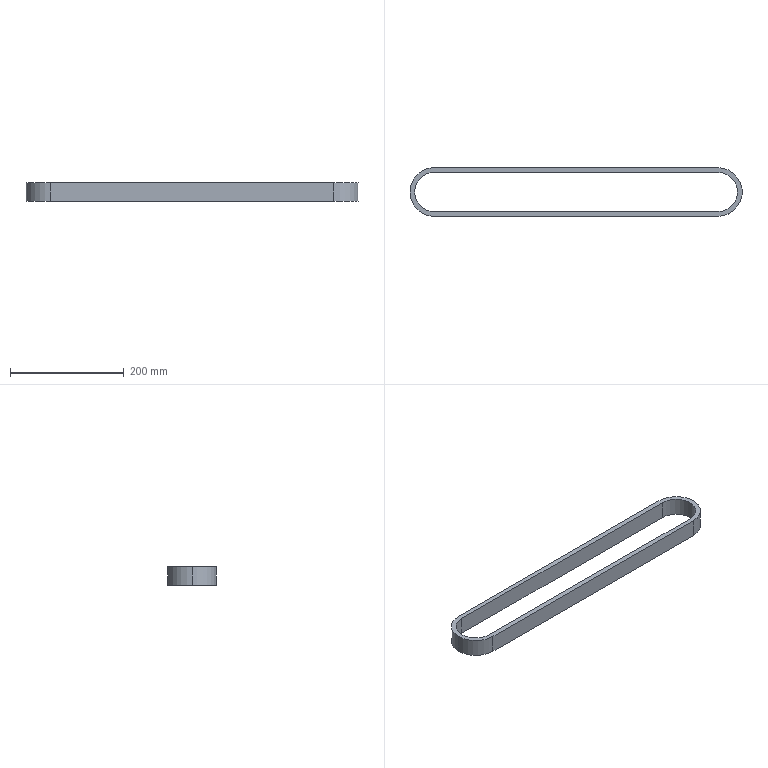Part | SolidWorks | features BaseBody 1 | 1 solid | 12 faces | box 583.72 x 85.72 x 32 mm | volume 329137 mm3 | cylinder 6 | plane 6 | commonest cylinder face diameters 69.12 x3 85.72 x3
STEP:
#1=CARTESIAN_POINT('',(0.,34.56,16.));
#2=VERTEX_POINT('',#1);
#3=CARTESIAN_POINT('',(-34.56,0.,16.));
#4=VERTEX_POINT('',#3);
#5=CARTESIAN_POINT('',(0.,0.,16.));
#6=DIRECTION('',(0.,0.,1.));
#7=DIRECTION('',(1.,0.,0.));
#8=AXIS2_PLACEMENT_3D('',#5,#6,#7);
#9=CIRCLE('',#8,34.56);
#10=EDGE_CURVE('',#2,#4,#9,.T.);
#11=ORIENTED_EDGE('',*,*,#10,.T.);
#12=CARTESIAN_POINT('',(-34.56,0.,-16.));
#13=VERTEX_POINT('',#12);
#14=CARTESIAN_POINT('',(-34.56,0.,16.));
#15=DIRECTION('',(0.,0.,-1.));
#16=VECTOR('',#15,1000.);
#17=LINE('',#14,#16);
#18=EDGE_CURVE('',#4,#13,#17,.T.);
#19=ORIENTED_EDGE('',*,*,#18,.T.);
#20=CARTESIAN_POINT('',(0.,34.56,-16.));
#21=VERTEX_POINT('',#20);
#22=CARTESIAN_POINT('',(0.,0.,-16.));
#23=DIRECTION('',(0.,0.,1.));
#24=DIRECTION('',(1.,0.,0.));
#25=AXIS2_PLACEMENT_3D('',#22,#23,#24);
#26=CIRCLE('',#25,34.56);
#27=EDGE_CURVE('',#21,#13,#26,.T.);
#28=ORIENTED_EDGE('',*,*,#27,.F.);
#29=CARTESIAN_POINT('',(0.,34.56,16.));
#30=DIRECTION('',(0.,0.,-1.));
#31=VECTOR('',#30,1000.);
#32=LINE('',#29,#31);
#33=EDGE_CURVE('',#2,#21,#32,.T.);
#34=ORIENTED_EDGE('',*,*,#33,.F.);
#35=EDGE_LOOP('',(#11,#19,#28,#34));
#36=FACE_OUTER_BOUND('',#35,.T.);
#37=CARTESIAN_POINT('',(0.,0.,16.));
#38=DIRECTION('',(0.,0.,-1.));
#39=DIRECTION('',(-1.,0.,0.));
#40=AXIS2_PLACEMENT_3D('',#37,#38,#39);
#41=CYLINDRICAL_SURFACE('',#40,34.56);
#42=ADVANCED_FACE('',(#36),#41,.F.);
#43=CARTESIAN_POINT('',(-42.86,0.,16.));
#44=VERTEX_POINT('',#43);
#45=CARTESIAN_POINT('',(0.,-42.86,16.));
#46=VERTEX_POINT('',#45);
#47=CARTESIAN_POINT('',(0.,0.,16.));
#48=DIRECTION('',(0.,0.,1.));
#49=DIRECTION('',(1.,0.,0.));
#50=AXIS2_PLACEMENT_3D('',#47,#48,#49);
#51=CIRCLE('',#50,42.86);
#52=EDGE_CURVE('',#44,#46,#51,.T.);
#53=ORIENTED_EDGE('',*,*,#52,.F.);
#54=CARTESIAN_POINT('',(-42.86,0.,-16.));
#55=VERTEX_POINT('',#54);
#56=CARTESIAN_POINT('',(-42.86,0.,16.));
#57=DIRECTION('',(0.,0.,-1.));
#58=VECTOR('',#57,1000.);
#59=LINE('',#56,#58);
#60=EDGE_CURVE('',#44,#55,#59,.T.);
#61=ORIENTED_EDGE('',*,*,#60,.T.);
#62=CARTESIAN_POINT('',(0.,-42.86,-16.));
#63=VERTEX_POINT('',#62);
#64=CARTESIAN_POINT('',(0.,0.,-16.));
#65=DIRECTION('',(0.,0.,1.));
#66=DIRECTION('',(1.,0.,0.));
#67=AXIS2_PLACEMENT_3D('',#64,#65,#66);
#68=CIRCLE('',#67,42.86);
#69=EDGE_CURVE('',#55,#63,#68,.T.);
#70=ORIENTED_EDGE('',*,*,#69,.T.);
#71=CARTESIAN_POINT('',(0.,-42.86,16.));
#72=DIRECTION('',(0.,0.,-1.));
#73=VECTOR('',#72,1000.);
#74=LINE('',#71,#73);
#75=EDGE_CURVE('',#46,#63,#74,.T.);
#76=ORIENTED_EDGE('',*,*,#75,.F.);
#77=EDGE_LOOP('',(#53,#61,#70,#76));
#78=FACE_OUTER_BOUND('',#77,.T.);
#79=CARTESIAN_POINT('',(0.,0.,16.));
#80=DIRECTION('',(0.,0.,-1.));
#81=DIRECTION('',(-1.,0.,0.));
#82=AXIS2_PLACEMENT_3D('',#79,#80,#81);
#83=CYLINDRICAL_SURFACE('',#82,42.86);
#84=ADVANCED_FACE('',(#78),#83,.T.);
#85=CARTESIAN_POINT('',(0.,42.86,16.));
#86=VERTEX_POINT('',#85);
#87=CARTESIAN_POINT('',(0.,0.,16.));
#88=DIRECTION('',(0.,0.,1.));
#89=DIRECTION('',(1.,0.,0.));
#90=AXIS2_PLACEMENT_3D('',#87,#88,#89);
#91=CIRCLE('',#90,42.86);
#92=EDGE_CURVE('',#86,#44,#91,.T.);
#93=ORIENTED_EDGE('',*,*,#92,.T.);
#94=ORIENTED_EDGE('',*,*,#52,.T.);
#95=CARTESIAN_POINT('',(498.,-42.86,16.));
#96=VERTEX_POINT('',#95);
#97=CARTESIAN_POINT('',(0.,-42.86,16.));
#98=DIRECTION('',(1.,0.,0.));
#99=VECTOR('',#98,1000.);
#100=LINE('',#97,#99);
#101=EDGE_CURVE('',#46,#96,#100,.T.);
#102=ORIENTED_EDGE('',*,*,#101,.T.);
#103=CARTESIAN_POINT('',(498.,42.86,16.));
#104=VERTEX_POINT('',#103);
#105=CARTESIAN_POINT('',(498.,0.,16.));
#106=DIRECTION('',(0.,0.,1.));
#107=DIRECTION('',(1.,0.,0.));
#108=AXIS2_PLACEMENT_3D('',#105,#106,#107);
#109=CIRCLE('',#108,42.86);
#110=EDGE_CURVE('',#96,#104,#109,.T.);
#111=ORIENTED_EDGE('',*,*,#110,.T.);
#112=CARTESIAN_POINT('',(0.,42.86,16.));
#113=DIRECTION('',(-1.,0.,0.));
#114=VECTOR('',#113,1000.);
#115=LINE('',#112,#114);
#116=EDGE_CURVE('',#104,#86,#115,.T.);
#117=ORIENTED_EDGE('',*,*,#116,.T.);
#118=EDGE_LOOP('',(#93,#94,#102,#111,#117));
#119=FACE_OUTER_BOUND('',#118,.T.);
#120=CARTESIAN_POINT('',(0.,-34.56,16.));
#121=VERTEX_POINT('',#120);
#122=CARTESIAN_POINT('',(498.,-34.56,16.));
#123=VERTEX_POINT('',#122);
#124=CARTESIAN_POINT('',(0.,-34.56,16.));
#125=DIRECTION('',(1.,0.,0.));
#126=VECTOR('',#125,1000.);
#127=LINE('',#124,#126);
#128=EDGE_CURVE('',#121,#123,#127,.T.);
#129=ORIENTED_EDGE('',*,*,#128,.F.);
#130=CARTESIAN_POINT('',(0.,0.,16.));
#131=DIRECTION('',(0.,0.,1.));
#132=DIRECTION('',(1.,0.,0.));
#133=AXIS2_PLACEMENT_3D('',#130,#131,#132);
#134=CIRCLE('',#133,34.56);
#135=EDGE_CURVE('',#4,#121,#134,.T.);
#136=ORIENTED_EDGE('',*,*,#135,.F.);
#137=ORIENTED_EDGE('',*,*,#10,.F.);
#138=CARTESIAN_POINT('',(498.,34.56,16.));
#139=VERTEX_POINT('',#138);
#140=CARTESIAN_POINT('',(0.,34.56,16.));
#141=DIRECTION('',(-1.,0.,0.));
#142=VECTOR('',#141,1000.);
#143=LINE('',#140,#142);
#144=EDGE_CURVE('',#139,#2,#143,.T.);
#145=ORIENTED_EDGE('',*,*,#144,.F.);
#146=CARTESIAN_POINT('',(498.,0.,16.));
#147=DIRECTION('',(0.,0.,1.));
#148=DIRECTION('',(1.,0.,0.));
#149=AXIS2_PLACEMENT_3D('',#146,#147,#148);
#150=CIRCLE('',#149,34.56);
#151=EDGE_CURVE('',#123,#139,#150,.T.);
#152=ORIENTED_EDGE('',*,*,#151,.F.);
#153=EDGE_LOOP('',(#129,#136,#137,#145,#152));
#154=FACE_BOUND('',#153,.T.);
#155=CARTESIAN_POINT('',(0.,0.,16.));
#156=DIRECTION('',(0.,0.,1.));
#157=DIRECTION('',(1.,0.,0.));
#158=AXIS2_PLACEMENT_3D('',#155,#156,#157);
#159=PLANE('',#158);
#160=ADVANCED_FACE('',(#119,#154),#159,.T.);
#161=CARTESIAN_POINT('',(0.,42.86,-16.));
#162=VERTEX_POINT('',#161);
#163=CARTESIAN_POINT('',(0.,0.,-16.));
#164=DIRECTION('',(0.,0.,1.));
#165=DIRECTION('',(1.,0.,0.));
#166=AXIS2_PLACEMENT_3D('',#163,#164,#165);
#167=CIRCLE('',#166,42.86);
#168=EDGE_CURVE('',#162,#55,#167,.T.);
#169=ORIENTED_EDGE('',*,*,#168,.F.);
#170=CARTESIAN_POINT('',(498.,42.86,-16.));
#171=VERTEX_POINT('',#170);
#172=CARTESIAN_POINT('',(0.,42.86,-16.));
#173=DIRECTION('',(-1.,0.,0.));
#174=VECTOR('',#173,1000.);
#175=LINE('',#172,#174);
#176=EDGE_CURVE('',#171,#162,#175,.T.);
#177=ORIENTED_EDGE('',*,*,#176,.F.);
#178=CARTESIAN_POINT('',(498.,-42.86,-16.));
#179=VERTEX_POINT('',#178);
#180=CARTESIAN_POINT('',(498.,0.,-16.));
#181=DIRECTION('',(0.,0.,1.));
#182=DIRECTION('',(1.,0.,0.));
#183=AXIS2_PLACEMENT_3D('',#180,#181,#182);
#184=CIRCLE('',#183,42.86);
#185=EDGE_CURVE('',#179,#171,#184,.T.);
#186=ORIENTED_EDGE('',*,*,#185,.F.);
#187=CARTESIAN_POINT('',(0.,-42.86,-16.));
#188=DIRECTION('',(1.,0.,0.));
#189=VECTOR('',#188,1000.);
#190=LINE('',#187,#189);
#191=EDGE_CURVE('',#63,#179,#190,.T.);
#192=ORIENTED_EDGE('',*,*,#191,.F.);
#193=ORIENTED_EDGE('',*,*,#69,.F.);
#194=EDGE_LOOP('',(#169,#177,#186,#192,#193));
#195=FACE_OUTER_BOUND('',#194,.T.);
#196=ORIENTED_EDGE('',*,*,#27,.T.);
#197=CARTESIAN_POINT('',(0.,-34.56,-16.));
#198=VERTEX_POINT('',#197);
#199=CARTESIAN_POINT('',(0.,0.,-16.));
#200=DIRECTION('',(0.,0.,1.));
#201=DIRECTION('',(1.,0.,0.));
#202=AXIS2_PLACEMENT_3D('',#199,#200,#201);
#203=CIRCLE('',#202,34.56);
#204=EDGE_CURVE('',#13,#198,#203,.T.);
#205=ORIENTED_EDGE('',*,*,#204,.T.);
#206=CARTESIAN_POINT('',(498.,-34.56,-16.));
#207=VERTEX_POINT('',#206);
#208=CARTESIAN_POINT('',(0.,-34.56,-16.));
#209=DIRECTION('',(1.,0.,0.));
#210=VECTOR('',#209,1000.);
#211=LINE('',#208,#210);
#212=EDGE_CURVE('',#198,#207,#211,.T.);
#213=ORIENTED_EDGE('',*,*,#212,.T.);
#214=CARTESIAN_POINT('',(498.,34.56,-16.));
#215=VERTEX_POINT('',#214);
#216=CARTESIAN_POINT('',(498.,0.,-16.));
#217=DIRECTION('',(0.,0.,1.));
#218=DIRECTION('',(1.,0.,0.));
#219=AXIS2_PLACEMENT_3D('',#216,#217,#218);
#220=CIRCLE('',#219,34.56);
#221=EDGE_CURVE('',#207,#215,#220,.T.);
#222=ORIENTED_EDGE('',*,*,#221,.T.);
#223=CARTESIAN_POINT('',(0.,34.56,-16.));
#224=DIRECTION('',(-1.,0.,0.));
#225=VECTOR('',#224,1000.);
#226=LINE('',#223,#225);
#227=EDGE_CURVE('',#215,#21,#226,.T.);
#228=ORIENTED_EDGE('',*,*,#227,.T.);
#229=EDGE_LOOP('',(#196,#205,#213,#222,#228));
#230=FACE_BOUND('',#229,.T.);
#231=CARTESIAN_POINT('',(0.,0.,-16.));
#232=DIRECTION('',(0.,0.,1.));
#233=DIRECTION('',(1.,0.,0.));
#234=AXIS2_PLACEMENT_3D('',#231,#232,#233);
#235=PLANE('',#234);
#236=ADVANCED_FACE('',(#195,#230),#235,.F.);
#237=ORIENTED_EDGE('',*,*,#60,.F.);
#238=ORIENTED_EDGE('',*,*,#92,.F.);
#239=CARTESIAN_POINT('',(0.,42.86,16.));
#240=DIRECTION('',(0.,0.,-1.));
#241=VECTOR('',#240,1000.);
#242=LINE('',#239,#241);
#243=EDGE_CURVE('',#86,#162,#242,.T.);
#244=ORIENTED_EDGE('',*,*,#243,.T.);
#245=ORIENTED_EDGE('',*,*,#168,.T.);
#246=EDGE_LOOP('',(#237,#238,#244,#245));
#247=FACE_OUTER_BOUND('',#246,.T.);
#248=CARTESIAN_POINT('',(0.,0.,16.));
#249=DIRECTION('',(0.,0.,-1.));
#250=DIRECTION('',(-1.,0.,0.));
#251=AXIS2_PLACEMENT_3D('',#248,#249,#250);
#252=CYLINDRICAL_SURFACE('',#251,42.86);
#253=ADVANCED_FACE('',(#247),#252,.T.);
#254=ORIENTED_EDGE('',*,*,#191,.T.);
#255=CARTESIAN_POINT('',(498.,-42.86,16.));
#256=DIRECTION('',(0.,0.,-1.));
#257=VECTOR('',#256,1000.);
#258=LINE('',#255,#257);
#259=EDGE_CURVE('',#96,#179,#258,.T.);
#260=ORIENTED_EDGE('',*,*,#259,.F.);
#261=ORIENTED_EDGE('',*,*,#101,.F.);
#262=ORIENTED_EDGE('',*,*,#75,.T.);
#263=EDGE_LOOP('',(#254,#260,#261,#262));
#264=FACE_OUTER_BOUND('',#263,.T.);
#265=CARTESIAN_POINT('',(0.,-42.86,16.));
#266=DIRECTION('',(0.,1.,0.));
#267=DIRECTION('',(0.,0.,1.));
#268=AXIS2_PLACEMENT_3D('',#265,#266,#267);
#269=PLANE('',#268);
#270=ADVANCED_FACE('',(#264),#269,.F.);
#271=ORIENTED_EDGE('',*,*,#185,.T.);
#272=CARTESIAN_POINT('',(498.,42.86,16.));
#273=DIRECTION('',(0.,0.,-1.));
#274=VECTOR('',#273,1000.);
#275=LINE('',#272,#274);
#276=EDGE_CURVE('',#104,#171,#275,.T.);
#277=ORIENTED_EDGE('',*,*,#276,.F.);
#278=ORIENTED_EDGE('',*,*,#110,.F.);
#279=ORIENTED_EDGE('',*,*,#259,.T.);
#280=EDGE_LOOP('',(#271,#277,#278,#279));
#281=FACE_OUTER_BOUND('',#280,.T.);
#282=CARTESIAN_POINT('',(498.,0.,16.));
#283=DIRECTION('',(0.,0.,-1.));
#284=DIRECTION('',(-1.,0.,0.));
#285=AXIS2_PLACEMENT_3D('',#282,#283,#284);
#286=CYLINDRICAL_SURFACE('',#285,42.86);
#287=ADVANCED_FACE('',(#281),#286,.T.);
#288=ORIENTED_EDGE('',*,*,#176,.T.);
#289=ORIENTED_EDGE('',*,*,#243,.F.);
#290=ORIENTED_EDGE('',*,*,#116,.F.);
#291=ORIENTED_EDGE('',*,*,#276,.T.);
#292=EDGE_LOOP('',(#288,#289,#290,#291));
#293=FACE_OUTER_BOUND('',#292,.T.);
#294=CARTESIAN_POINT('',(0.,42.86,16.));
#295=DIRECTION('',(0.,-1.,0.));
#296=DIRECTION('',(0.,0.,-1.));
#297=AXIS2_PLACEMENT_3D('',#294,#295,#296);
#298=PLANE('',#297);
#299=ADVANCED_FACE('',(#293),#298,.F.);
#300=ORIENTED_EDGE('',*,*,#18,.F.);
#301=ORIENTED_EDGE('',*,*,#135,.T.);
#302=CARTESIAN_POINT('',(0.,-34.56,16.));
#303=DIRECTION('',(0.,0.,-1.));
#304=VECTOR('',#303,1000.);
#305=LINE('',#302,#304);
#306=EDGE_CURVE('',#121,#198,#305,.T.);
#307=ORIENTED_EDGE('',*,*,#306,.T.);
#308=ORIENTED_EDGE('',*,*,#204,.F.);
#309=EDGE_LOOP('',(#300,#301,#307,#308));
#310=FACE_OUTER_BOUND('',#309,.T.);
#311=CARTESIAN_POINT('',(0.,0.,16.));
#312=DIRECTION('',(0.,0.,-1.));
#313=DIRECTION('',(-1.,0.,0.));
#314=AXIS2_PLACEMENT_3D('',#311,#312,#313);
#315=CYLINDRICAL_SURFACE('',#314,34.56);
#316=ADVANCED_FACE('',(#310),#315,.F.);
#317=ORIENTED_EDGE('',*,*,#212,.F.);
#318=ORIENTED_EDGE('',*,*,#306,.F.);
#319=ORIENTED_EDGE('',*,*,#128,.T.);
#320=CARTESIAN_POINT('',(498.,-34.56,16.));
#321=DIRECTION('',(0.,0.,-1.));
#322=VECTOR('',#321,1000.);
#323=LINE('',#320,#322);
#324=EDGE_CURVE('',#123,#207,#323,.T.);
#325=ORIENTED_EDGE('',*,*,#324,.T.);
#326=EDGE_LOOP('',(#317,#318,#319,#325));
#327=FACE_OUTER_BOUND('',#326,.T.);
#328=CARTESIAN_POINT('',(0.,-34.56,16.));
#329=DIRECTION('',(0.,1.,0.));
#330=DIRECTION('',(0.,0.,1.));
#331=AXIS2_PLACEMENT_3D('',#328,#329,#330);
#332=PLANE('',#331);
#333=ADVANCED_FACE('',(#327),#332,.T.);
#334=ORIENTED_EDGE('',*,*,#221,.F.);
#335=ORIENTED_EDGE('',*,*,#324,.F.);
#336=ORIENTED_EDGE('',*,*,#151,.T.);
#337=CARTESIAN_POINT('',(498.,34.56,16.));
#338=DIRECTION('',(0.,0.,-1.));
#339=VECTOR('',#338,1000.);
#340=LINE('',#337,#339);
#341=EDGE_CURVE('',#139,#215,#340,.T.);
#342=ORIENTED_EDGE('',*,*,#341,.T.);
#343=EDGE_LOOP('',(#334,#335,#336,#342));
#344=FACE_OUTER_BOUND('',#343,.T.);
#345=CARTESIAN_POINT('',(498.,0.,16.));
#346=DIRECTION('',(0.,0.,-1.));
#347=DIRECTION('',(-1.,0.,0.));
#348=AXIS2_PLACEMENT_3D('',#345,#346,#347);
#349=CYLINDRICAL_SURFACE('',#348,34.56);
#350=ADVANCED_FACE('',(#344),#349,.F.);
#351=ORIENTED_EDGE('',*,*,#227,.F.);
#352=ORIENTED_EDGE('',*,*,#341,.F.);
#353=ORIENTED_EDGE('',*,*,#144,.T.);
#354=ORIENTED_EDGE('',*,*,#33,.T.);
#355=EDGE_LOOP('',(#351,#352,#353,#354));
#356=FACE_OUTER_BOUND('',#355,.T.);
#357=CARTESIAN_POINT('',(0.,34.56,16.));
#358=DIRECTION('',(0.,-1.,0.));
#359=DIRECTION('',(0.,0.,-1.));
#360=AXIS2_PLACEMENT_3D('',#357,#358,#359);
#361=PLANE('',#360);
#362=ADVANCED_FACE('',(#356),#361,.T.);
#363=CLOSED_SHELL('',(#42,#84,#160,#236,#253,#270,#287,#299,#316,#333,#350,#362));
#364=MANIFOLD_SOLID_BREP('',#363);
#365=CARTESIAN_POINT('',(0.,0.,0.));
#366=DIRECTION('',(0.,0.,1.));
#367=DIRECTION('',(1.,0.,0.));
#368=AXIS2_PLACEMENT_3D('',#365,#366,#367);
#369=(LENGTH_UNIT()NAMED_UNIT(*)SI_UNIT(.MILLI.,.METRE.));
#370=UNCERTAINTY_MEASURE_WITH_UNIT(LENGTH_MEASURE(0.00001),#369,'','');
#371=(NAMED_UNIT(*)PLANE_ANGLE_UNIT()SI_UNIT($,.RADIAN.));
#372=(NAMED_UNIT(*)SI_UNIT($,.STERADIAN.)SOLID_ANGLE_UNIT());
#373=(GEOMETRIC_REPRESENTATION_CONTEXT(3)GLOBAL_UNCERTAINTY_ASSIGNED_CONTEXT((#370))GLOBAL_UNIT_ASSIGNED_CONTEXT((#369,#371,#372))REPRESENTATION_CONTEXT('',''));
#374=ADVANCED_BREP_SHAPE_REPRESENTATION('',(#364,#368),#373);